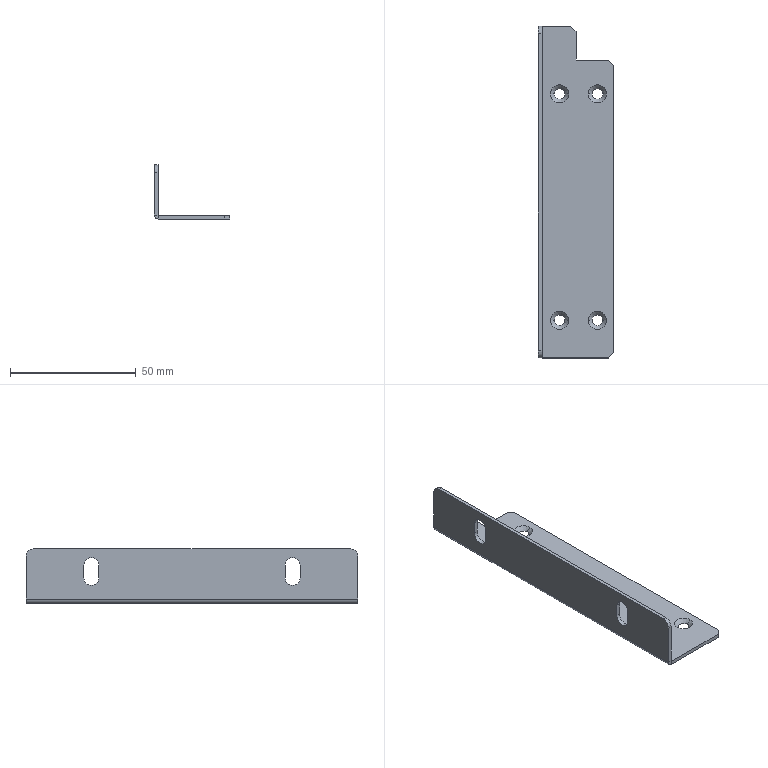Part | SolidWorks | features ICE 3, CornerTrim 2, Chamfer 1, EdgeFlange 1, FlatPattern 1, SMBaseFlange 1, SheetMetal 1 | 1 solid | 39 faces | box 30 x 132 x 21.5 mm | volume 9178 mm3 | plane 21 | cylinder 10 | cone 8 | commonest cylinder face diameters 6 x8 0.2 x1 3.2 x1
STEP:
#1=CARTESIAN_POINT('',(-8.6,39.,-1.5));
#2=VERTEX_POINT('',#1);
#3=CARTESIAN_POINT('',(-4.4,39.,-1.5));
#4=VERTEX_POINT('',#3);
#5=CARTESIAN_POINT('',(-6.5,39.,-1.5));
#6=DIRECTION('',(0.,0.,1.));
#7=DIRECTION('',(1.,0.,0.));
#8=AXIS2_PLACEMENT_3D('',#5,#6,#7);
#9=CIRCLE('',#8,2.1);
#10=EDGE_CURVE('',#2,#4,#9,.T.);
#11=ORIENTED_EDGE('',*,*,#10,.F.);
#12=CARTESIAN_POINT('',(-10.1,39.,0.));
#13=VERTEX_POINT('',#12);
#14=CARTESIAN_POINT('',(-8.6,39.,-1.5));
#15=DIRECTION('',(-0.7071,0.,0.7071));
#16=VECTOR('',#15,1000.);
#17=LINE('',#14,#16);
#18=EDGE_CURVE('',#2,#13,#17,.T.);
#19=ORIENTED_EDGE('',*,*,#18,.T.);
#20=CARTESIAN_POINT('',(-2.9,39.,0.));
#21=VERTEX_POINT('',#20);
#22=CARTESIAN_POINT('',(-6.5,39.,0.));
#23=DIRECTION('',(0.,0.,-1.));
#24=DIRECTION('',(1.,0.,0.));
#25=AXIS2_PLACEMENT_3D('',#22,#23,#24);
#26=CIRCLE('',#25,3.6);
#27=EDGE_CURVE('',#21,#13,#26,.T.);
#28=ORIENTED_EDGE('',*,*,#27,.F.);
#29=CARTESIAN_POINT('',(-4.4,39.,-1.5));
#30=DIRECTION('',(0.7071,0.,0.7071));
#31=VECTOR('',#30,1000.);
#32=LINE('',#29,#31);
#33=EDGE_CURVE('',#4,#21,#32,.T.);
#34=ORIENTED_EDGE('',*,*,#33,.F.);
#35=EDGE_LOOP('',(#11,#19,#28,#34));
#36=FACE_OUTER_BOUND('',#35,.T.);
#37=CARTESIAN_POINT('',(-6.5,39.,-1.5));
#38=DIRECTION('',(0.,0.,1.));
#39=DIRECTION('',(1.,0.,0.));
#40=AXIS2_PLACEMENT_3D('',#37,#38,#39);
#41=CONICAL_SURFACE('',#40,2.1,0.7854);
#42=ADVANCED_FACE('',(#36),#41,.F.);
#43=CARTESIAN_POINT('',(6.4,39.,-1.5));
#44=VERTEX_POINT('',#43);
#45=CARTESIAN_POINT('',(10.6,39.,-1.5));
#46=VERTEX_POINT('',#45);
#47=CARTESIAN_POINT('',(8.5,39.,-1.5));
#48=DIRECTION('',(0.,0.,1.));
#49=DIRECTION('',(1.,0.,0.));
#50=AXIS2_PLACEMENT_3D('',#47,#48,#49);
#51=CIRCLE('',#50,2.1);
#52=EDGE_CURVE('',#44,#46,#51,.T.);
#53=ORIENTED_EDGE('',*,*,#52,.F.);
#54=CARTESIAN_POINT('',(4.9,39.,0.));
#55=VERTEX_POINT('',#54);
#56=CARTESIAN_POINT('',(6.4,39.,-1.5));
#57=DIRECTION('',(-0.7071,0.,0.7071));
#58=VECTOR('',#57,1000.);
#59=LINE('',#56,#58);
#60=EDGE_CURVE('',#44,#55,#59,.T.);
#61=ORIENTED_EDGE('',*,*,#60,.T.);
#62=CARTESIAN_POINT('',(12.1,39.,0.));
#63=VERTEX_POINT('',#62);
#64=CARTESIAN_POINT('',(8.5,39.,0.));
#65=DIRECTION('',(0.,0.,-1.));
#66=DIRECTION('',(1.,0.,0.));
#67=AXIS2_PLACEMENT_3D('',#64,#65,#66);
#68=CIRCLE('',#67,3.6);
#69=EDGE_CURVE('',#63,#55,#68,.T.);
#70=ORIENTED_EDGE('',*,*,#69,.F.);
#71=CARTESIAN_POINT('',(10.6,39.,-1.5));
#72=DIRECTION('',(0.7071,0.,0.7071));
#73=VECTOR('',#72,1000.);
#74=LINE('',#71,#73);
#75=EDGE_CURVE('',#46,#63,#74,.T.);
#76=ORIENTED_EDGE('',*,*,#75,.F.);
#77=EDGE_LOOP('',(#53,#61,#70,#76));
#78=FACE_OUTER_BOUND('',#77,.T.);
#79=CARTESIAN_POINT('',(8.5,39.,-1.5));
#80=DIRECTION('',(0.,0.,1.));
#81=DIRECTION('',(1.,0.,0.));
#82=AXIS2_PLACEMENT_3D('',#79,#80,#81);
#83=CONICAL_SURFACE('',#82,2.1,0.7854);
#84=ADVANCED_FACE('',(#78),#83,.F.);
#85=CARTESIAN_POINT('',(6.4,-51.,-1.5));
#86=VERTEX_POINT('',#85);
#87=CARTESIAN_POINT('',(10.6,-51.,-1.5));
#88=VERTEX_POINT('',#87);
#89=CARTESIAN_POINT('',(8.5,-51.,-1.5));
#90=DIRECTION('',(0.,0.,1.));
#91=DIRECTION('',(1.,0.,0.));
#92=AXIS2_PLACEMENT_3D('',#89,#90,#91);
#93=CIRCLE('',#92,2.1);
#94=EDGE_CURVE('',#86,#88,#93,.T.);
#95=ORIENTED_EDGE('',*,*,#94,.F.);
#96=CARTESIAN_POINT('',(4.9,-51.,0.));
#97=VERTEX_POINT('',#96);
#98=CARTESIAN_POINT('',(6.4,-51.,-1.5));
#99=DIRECTION('',(-0.7071,0.,0.7071));
#100=VECTOR('',#99,1000.);
#101=LINE('',#98,#100);
#102=EDGE_CURVE('',#86,#97,#101,.T.);
#103=ORIENTED_EDGE('',*,*,#102,.T.);
#104=CARTESIAN_POINT('',(12.1,-51.,0.));
#105=VERTEX_POINT('',#104);
#106=CARTESIAN_POINT('',(8.5,-51.,0.));
#107=DIRECTION('',(0.,0.,-1.));
#108=DIRECTION('',(1.,0.,0.));
#109=AXIS2_PLACEMENT_3D('',#106,#107,#108);
#110=CIRCLE('',#109,3.6);
#111=EDGE_CURVE('',#105,#97,#110,.T.);
#112=ORIENTED_EDGE('',*,*,#111,.F.);
#113=CARTESIAN_POINT('',(10.6,-51.,-1.5));
#114=DIRECTION('',(0.7071,0.,0.7071));
#115=VECTOR('',#114,1000.);
#116=LINE('',#113,#115);
#117=EDGE_CURVE('',#88,#105,#116,.T.);
#118=ORIENTED_EDGE('',*,*,#117,.F.);
#119=EDGE_LOOP('',(#95,#103,#112,#118));
#120=FACE_OUTER_BOUND('',#119,.T.);
#121=CARTESIAN_POINT('',(8.5,-51.,-1.5));
#122=DIRECTION('',(0.,0.,1.));
#123=DIRECTION('',(1.,0.,0.));
#124=AXIS2_PLACEMENT_3D('',#121,#122,#123);
#125=CONICAL_SURFACE('',#124,2.1,0.7854);
#126=ADVANCED_FACE('',(#120),#125,.F.);
#127=CARTESIAN_POINT('',(-8.6,-51.,-1.5));
#128=VERTEX_POINT('',#127);
#129=CARTESIAN_POINT('',(-4.4,-51.,-1.5));
#130=VERTEX_POINT('',#129);
#131=CARTESIAN_POINT('',(-6.5,-51.,-1.5));
#132=DIRECTION('',(0.,0.,1.));
#133=DIRECTION('',(1.,0.,0.));
#134=AXIS2_PLACEMENT_3D('',#131,#132,#133);
#135=CIRCLE('',#134,2.1);
#136=EDGE_CURVE('',#128,#130,#135,.T.);
#137=ORIENTED_EDGE('',*,*,#136,.F.);
#138=CARTESIAN_POINT('',(-10.1,-51.,0.));
#139=VERTEX_POINT('',#138);
#140=CARTESIAN_POINT('',(-8.6,-51.,-1.5));
#141=DIRECTION('',(-0.7071,0.,0.7071));
#142=VECTOR('',#141,1000.);
#143=LINE('',#140,#142);
#144=EDGE_CURVE('',#128,#139,#143,.T.);
#145=ORIENTED_EDGE('',*,*,#144,.T.);
#146=CARTESIAN_POINT('',(-2.9,-51.,0.));
#147=VERTEX_POINT('',#146);
#148=CARTESIAN_POINT('',(-6.5,-51.,0.));
#149=DIRECTION('',(0.,0.,-1.));
#150=DIRECTION('',(1.,0.,0.));
#151=AXIS2_PLACEMENT_3D('',#148,#149,#150);
#152=CIRCLE('',#151,3.6);
#153=EDGE_CURVE('',#147,#139,#152,.T.);
#154=ORIENTED_EDGE('',*,*,#153,.F.);
#155=CARTESIAN_POINT('',(-4.4,-51.,-1.5));
#156=DIRECTION('',(0.7071,0.,0.7071));
#157=VECTOR('',#156,1000.);
#158=LINE('',#155,#157);
#159=EDGE_CURVE('',#130,#147,#158,.T.);
#160=ORIENTED_EDGE('',*,*,#159,.F.);
#161=EDGE_LOOP('',(#137,#145,#154,#160));
#162=FACE_OUTER_BOUND('',#161,.T.);
#163=CARTESIAN_POINT('',(-6.5,-51.,-1.5));
#164=DIRECTION('',(0.,0.,1.));
#165=DIRECTION('',(1.,0.,0.));
#166=AXIS2_PLACEMENT_3D('',#163,#164,#165);
#167=CONICAL_SURFACE('',#166,2.1,0.7854);
#168=ADVANCED_FACE('',(#162),#167,.F.);
#169=CARTESIAN_POINT('',(-13.5,43.,13.5));
#170=VERTEX_POINT('',#169);
#171=CARTESIAN_POINT('',(-13.5,40.,16.5));
#172=VERTEX_POINT('',#171);
#173=CARTESIAN_POINT('',(-13.5,40.,13.5));
#174=DIRECTION('',(1.,0.,0.));
#175=DIRECTION('',(0.,0.,-1.));
#176=AXIS2_PLACEMENT_3D('',#173,#174,#175);
#177=CIRCLE('',#176,3.);
#178=EDGE_CURVE('',#170,#172,#177,.T.);
#179=ORIENTED_EDGE('',*,*,#178,.T.);
#180=CARTESIAN_POINT('',(-15.,40.,16.5));
#181=VERTEX_POINT('',#180);
#182=CARTESIAN_POINT('',(-5.,40.,16.5));
#183=DIRECTION('',(-1.,0.,0.));
#184=VECTOR('',#183,1000.);
#185=LINE('',#182,#184);
#186=EDGE_CURVE('',#172,#181,#185,.T.);
#187=ORIENTED_EDGE('',*,*,#186,.T.);
#188=CARTESIAN_POINT('',(-15.,43.,13.5));
#189=VERTEX_POINT('',#188);
#190=CARTESIAN_POINT('',(-15.,40.,13.5));
#191=DIRECTION('',(-1.,0.,0.));
#192=DIRECTION('',(0.,0.,1.));
#193=AXIS2_PLACEMENT_3D('',#190,#191,#192);
#194=CIRCLE('',#193,3.);
#195=EDGE_CURVE('',#181,#189,#194,.T.);
#196=ORIENTED_EDGE('',*,*,#195,.T.);
#197=CARTESIAN_POINT('',(-5.,43.,13.5));
#198=DIRECTION('',(-1.,0.,0.));
#199=VECTOR('',#198,1000.);
#200=LINE('',#197,#199);
#201=EDGE_CURVE('',#170,#189,#200,.T.);
#202=ORIENTED_EDGE('',*,*,#201,.F.);
#203=EDGE_LOOP('',(#179,#187,#196,#202));
#204=FACE_OUTER_BOUND('',#203,.T.);
#205=CARTESIAN_POINT('',(-5.,40.,13.5));
#206=DIRECTION('',(-1.,0.,0.));
#207=DIRECTION('',(0.,0.,1.));
#208=AXIS2_PLACEMENT_3D('',#205,#206,#207);
#209=CYLINDRICAL_SURFACE('',#208,3.);
#210=ADVANCED_FACE('',(#204),#209,.F.);
#211=CARTESIAN_POINT('',(-13.5,-37.,13.5));
#212=VERTEX_POINT('',#211);
#213=CARTESIAN_POINT('',(-13.5,-40.,16.5));
#214=VERTEX_POINT('',#213);
#215=CARTESIAN_POINT('',(-13.5,-40.,13.5));
#216=DIRECTION('',(1.,0.,0.));
#217=DIRECTION('',(0.,0.,-1.));
#218=AXIS2_PLACEMENT_3D('',#215,#216,#217);
#219=CIRCLE('',#218,3.);
#220=EDGE_CURVE('',#212,#214,#219,.T.);
#221=ORIENTED_EDGE('',*,*,#220,.T.);
#222=CARTESIAN_POINT('',(-15.,-40.,16.5));
#223=VERTEX_POINT('',#222);
#224=CARTESIAN_POINT('',(-5.,-40.,16.5));
#225=DIRECTION('',(-1.,0.,0.));
#226=VECTOR('',#225,1000.);
#227=LINE('',#224,#226);
#228=EDGE_CURVE('',#214,#223,#227,.T.);
#229=ORIENTED_EDGE('',*,*,#228,.T.);
#230=CARTESIAN_POINT('',(-15.,-37.,13.5));
#231=VERTEX_POINT('',#230);
#232=CARTESIAN_POINT('',(-15.,-40.,13.5));
#233=DIRECTION('',(-1.,0.,0.));
#234=DIRECTION('',(0.,0.,1.));
#235=AXIS2_PLACEMENT_3D('',#232,#233,#234);
#236=CIRCLE('',#235,3.);
#237=EDGE_CURVE('',#223,#231,#236,.T.);
#238=ORIENTED_EDGE('',*,*,#237,.T.);
#239=CARTESIAN_POINT('',(-5.,-37.,13.5));
#240=DIRECTION('',(-1.,0.,0.));
#241=VECTOR('',#240,1000.);
#242=LINE('',#239,#241);
#243=EDGE_CURVE('',#212,#231,#242,.T.);
#244=ORIENTED_EDGE('',*,*,#243,.F.);
#245=EDGE_LOOP('',(#221,#229,#238,#244));
#246=FACE_OUTER_BOUND('',#245,.T.);
#247=CARTESIAN_POINT('',(-5.,-40.,13.5));
#248=DIRECTION('',(-1.,0.,0.));
#249=DIRECTION('',(0.,0.,1.));
#250=AXIS2_PLACEMENT_3D('',#247,#248,#249);
#251=CYLINDRICAL_SURFACE('',#250,3.);
#252=ADVANCED_FACE('',(#246),#251,.F.);
#253=CARTESIAN_POINT('',(-13.4,-66.,-1.5));
#254=VERTEX_POINT('',#253);
#255=CARTESIAN_POINT('',(13.,-66.,-1.5));
#256=VERTEX_POINT('',#255);
#257=CARTESIAN_POINT('',(-15.,-66.,-1.5));
#258=DIRECTION('',(1.,0.,0.));
#259=VECTOR('',#258,1000.);
#260=LINE('',#257,#259);
#261=EDGE_CURVE('',#254,#256,#260,.T.);
#262=ORIENTED_EDGE('',*,*,#261,.T.);
#263=CARTESIAN_POINT('',(13.,-66.,0.));
#264=VERTEX_POINT('',#263);
#265=CARTESIAN_POINT('',(13.,-66.,-1.5));
#266=DIRECTION('',(0.,0.,1.));
#267=VECTOR('',#266,1000.);
#268=LINE('',#265,#267);
#269=EDGE_CURVE('',#256,#264,#268,.T.);
#270=ORIENTED_EDGE('',*,*,#269,.T.);
#271=CARTESIAN_POINT('',(-13.4,-66.,0.));
#272=VERTEX_POINT('',#271);
#273=CARTESIAN_POINT('',(-15.,-66.,0.));
#274=DIRECTION('',(1.,0.,0.));
#275=VECTOR('',#274,1000.);
#276=LINE('',#273,#275);
#277=EDGE_CURVE('',#272,#264,#276,.T.);
#278=ORIENTED_EDGE('',*,*,#277,.F.);
#279=CARTESIAN_POINT('',(-13.4,-66.,0.));
#280=DIRECTION('',(0.,0.,-1.));
#281=VECTOR('',#280,1000.);
#282=LINE('',#279,#281);
#283=EDGE_CURVE('',#272,#254,#282,.T.);
#284=ORIENTED_EDGE('',*,*,#283,.T.);
#285=EDGE_LOOP('',(#262,#270,#278,#284));
#286=FACE_OUTER_BOUND('',#285,.T.);
#287=CARTESIAN_POINT('',(-15.,-66.,-1.5));
#288=DIRECTION('',(0.,-1.,0.));
#289=DIRECTION('',(0.,0.,-1.));
#290=AXIS2_PLACEMENT_3D('',#287,#288,#289);
#291=PLANE('',#290);
#292=ADVANCED_FACE('',(#286),#291,.T.);
#293=CARTESIAN_POINT('',(-6.5,-51.,-1.5));
#294=DIRECTION('',(0.,0.,1.));
#295=DIRECTION('',(1.,0.,0.));
#296=AXIS2_PLACEMENT_3D('',#293,#294,#295);
#297=CIRCLE('',#296,2.1);
#298=EDGE_CURVE('',#130,#128,#297,.T.);
#299=ORIENTED_EDGE('',*,*,#298,.T.);
#300=ORIENTED_EDGE('',*,*,#136,.T.);
#301=EDGE_LOOP('',(#299,#300));
#302=FACE_BOUND('',#301,.T.);
#303=CARTESIAN_POINT('',(8.5,-51.,-1.5));
#304=DIRECTION('',(0.,0.,1.));
#305=DIRECTION('',(1.,0.,0.));
#306=AXIS2_PLACEMENT_3D('',#303,#304,#305);
#307=CIRCLE('',#306,2.1);
#308=EDGE_CURVE('',#88,#86,#307,.T.);
#309=ORIENTED_EDGE('',*,*,#308,.T.);
#310=ORIENTED_EDGE('',*,*,#94,.T.);
#311=EDGE_LOOP('',(#309,#310));
#312=FACE_BOUND('',#311,.T.);
#313=CARTESIAN_POINT('',(8.5,39.,-1.5));
#314=DIRECTION('',(0.,0.,1.));
#315=DIRECTION('',(1.,0.,0.));
#316=AXIS2_PLACEMENT_3D('',#313,#314,#315);
#317=CIRCLE('',#316,2.1);
#318=EDGE_CURVE('',#46,#44,#317,.T.);
#319=ORIENTED_EDGE('',*,*,#318,.T.);
#320=ORIENTED_EDGE('',*,*,#52,.T.);
#321=EDGE_LOOP('',(#319,#320));
#322=FACE_BOUND('',#321,.T.);
#323=CARTESIAN_POINT('',(-6.5,39.,-1.5));
#324=DIRECTION('',(0.,0.,1.));
#325=DIRECTION('',(1.,0.,0.));
#326=AXIS2_PLACEMENT_3D('',#323,#324,#325);
#327=CIRCLE('',#326,2.1);
#328=EDGE_CURVE('',#4,#2,#327,.T.);
#329=ORIENTED_EDGE('',*,*,#328,.T.);
#330=ORIENTED_EDGE('',*,*,#10,.T.);
#331=EDGE_LOOP('',(#329,#330));
#332=FACE_BOUND('',#331,.T.);
#333=CARTESIAN_POINT('',(0.,52.5,-1.5));
#334=VERTEX_POINT('',#333);
#335=CARTESIAN_POINT('',(13.,52.5,-1.5));
#336=VERTEX_POINT('',#335);
#337=CARTESIAN_POINT('',(0.,52.5,-1.5));
#338=DIRECTION('',(1.,0.,0.));
#339=VECTOR('',#338,1000.);
#340=LINE('',#337,#339);
#341=EDGE_CURVE('',#334,#336,#340,.T.);
#342=ORIENTED_EDGE('',*,*,#341,.T.);
#343=CARTESIAN_POINT('',(15.,50.5,-1.5));
#344=VERTEX_POINT('',#343);
#345=CARTESIAN_POINT('',(15.,50.5,-1.5));
#346=DIRECTION('',(0.7071,-0.7071,0.));
#347=VECTOR('',#346,1000.);
#348=LINE('',#345,#347);
#349=EDGE_CURVE('',#336,#344,#348,.T.);
#350=ORIENTED_EDGE('',*,*,#349,.T.);
#351=CARTESIAN_POINT('',(15.,-64.,-1.5));
#352=VERTEX_POINT('',#351);
#353=CARTESIAN_POINT('',(15.,66.,-1.5));
#354=DIRECTION('',(0.,1.,0.));
#355=VECTOR('',#354,1000.);
#356=LINE('',#353,#355);
#357=EDGE_CURVE('',#352,#344,#356,.T.);
#358=ORIENTED_EDGE('',*,*,#357,.F.);
#359=CARTESIAN_POINT('',(13.,-66.,-1.5));
#360=DIRECTION('',(-0.7071,-0.7071,0.));
#361=VECTOR('',#360,1000.);
#362=LINE('',#359,#361);
#363=EDGE_CURVE('',#352,#256,#362,.T.);
#364=ORIENTED_EDGE('',*,*,#363,.T.);
#365=ORIENTED_EDGE('',*,*,#261,.F.);
#366=CARTESIAN_POINT('',(-13.4,66.,-1.5));
#367=VERTEX_POINT('',#366);
#368=CARTESIAN_POINT('',(-13.4,-66.,-1.5));
#369=DIRECTION('',(0.,1.,0.));
#370=VECTOR('',#369,1000.);
#371=LINE('',#368,#370);
#372=EDGE_CURVE('',#254,#367,#371,.T.);
#373=ORIENTED_EDGE('',*,*,#372,.T.);
#374=CARTESIAN_POINT('',(-2.,66.,-1.5));
#375=VERTEX_POINT('',#374);
#376=CARTESIAN_POINT('',(-15.,66.,-1.5));
#377=DIRECTION('',(-1.,0.,0.));
#378=VECTOR('',#377,1000.);
#379=LINE('',#376,#378);
#380=EDGE_CURVE('',#375,#367,#379,.T.);
#381=ORIENTED_EDGE('',*,*,#380,.F.);
#382=CARTESIAN_POINT('',(0.,64.,-1.5));
#383=VERTEX_POINT('',#382);
#384=CARTESIAN_POINT('',(0.,64.,-1.5));
#385=DIRECTION('',(0.7071,-0.7071,0.));
#386=VECTOR('',#385,1000.);
#387=LINE('',#384,#386);
#388=EDGE_CURVE('',#375,#383,#387,.T.);
#389=ORIENTED_EDGE('',*,*,#388,.T.);
#390=CARTESIAN_POINT('',(0.,0.,-1.5));
#391=DIRECTION('',(0.,-1.,0.));
#392=VECTOR('',#391,1000.);
#393=LINE('',#390,#392);
#394=EDGE_CURVE('',#383,#334,#393,.T.);
#395=ORIENTED_EDGE('',*,*,#394,.T.);
#396=EDGE_LOOP('',(#342,#350,#358,#364,#365,#373,#381,#389,#395));
#397=FACE_OUTER_BOUND('',#396,.T.);
#398=CARTESIAN_POINT('',(0.,0.,-1.5));
#399=DIRECTION('',(0.,0.,1.));
#400=DIRECTION('',(1.,0.,0.));
#401=AXIS2_PLACEMENT_3D('',#398,#399,#400);
#402=PLANE('',#401);
#403=ADVANCED_FACE('',(#302,#312,#322,#332,#397),#402,.F.);
#404=ORIENTED_EDGE('',*,*,#153,.T.);
#405=CARTESIAN_POINT('',(-6.5,-51.,0.));
#406=DIRECTION('',(0.,0.,-1.));
#407=DIRECTION('',(1.,0.,0.));
#408=AXIS2_PLACEMENT_3D('',#405,#406,#407);
#409=CIRCLE('',#408,3.6);
#410=EDGE_CURVE('',#139,#147,#409,.T.);
#411=ORIENTED_EDGE('',*,*,#410,.T.);
#412=EDGE_LOOP('',(#404,#411));
#413=FACE_BOUND('',#412,.T.);
#414=ORIENTED_EDGE('',*,*,#111,.T.);
#415=CARTESIAN_POINT('',(8.5,-51.,0.));
#416=DIRECTION('',(0.,0.,-1.));
#417=DIRECTION('',(1.,0.,0.));
#418=AXIS2_PLACEMENT_3D('',#415,#416,#417);
#419=CIRCLE('',#418,3.6);
#420=EDGE_CURVE('',#97,#105,#419,.T.);
#421=ORIENTED_EDGE('',*,*,#420,.T.);
#422=EDGE_LOOP('',(#414,#421));
#423=FACE_BOUND('',#422,.T.);
#424=ORIENTED_EDGE('',*,*,#69,.T.);
#425=CARTESIAN_POINT('',(8.5,39.,0.));
#426=DIRECTION('',(0.,0.,-1.));
#427=DIRECTION('',(1.,0.,0.));
#428=AXIS2_PLACEMENT_3D('',#425,#426,#427);
#429=CIRCLE('',#428,3.6);
#430=EDGE_CURVE('',#55,#63,#429,.T.);
#431=ORIENTED_EDGE('',*,*,#430,.T.);
#432=EDGE_LOOP('',(#424,#431));
#433=FACE_BOUND('',#432,.T.);
#434=ORIENTED_EDGE('',*,*,#27,.T.);
#435=CARTESIAN_POINT('',(-6.5,39.,0.));
#436=DIRECTION('',(0.,0.,-1.));
#437=DIRECTION('',(1.,0.,0.));
#438=AXIS2_PLACEMENT_3D('',#435,#436,#437);
#439=CIRCLE('',#438,3.6);
#440=EDGE_CURVE('',#13,#21,#439,.T.);
#441=ORIENTED_EDGE('',*,*,#440,.T.);
#442=EDGE_LOOP('',(#434,#441));
#443=FACE_BOUND('',#442,.T.);
#444=CARTESIAN_POINT('',(15.,-64.,0.));
#445=VERTEX_POINT('',#444);
#446=CARTESIAN_POINT('',(15.,50.5,0.));
#447=VERTEX_POINT('',#446);
#448=CARTESIAN_POINT('',(15.,66.,0.));
#449=DIRECTION('',(0.,1.,0.));
#450=VECTOR('',#449,1000.);
#451=LINE('',#448,#450);
#452=EDGE_CURVE('',#445,#447,#451,.T.);
#453=ORIENTED_EDGE('',*,*,#452,.T.);
#454=CARTESIAN_POINT('',(13.,52.5,0.));
#455=VERTEX_POINT('',#454);
#456=CARTESIAN_POINT('',(32.75,32.75,0.));
#457=DIRECTION('',(-0.7071,0.7071,0.));
#458=VECTOR('',#457,1000.);
#459=LINE('',#456,#458);
#460=EDGE_CURVE('',#447,#455,#459,.T.);
#461=ORIENTED_EDGE('',*,*,#460,.T.);
#462=CARTESIAN_POINT('',(0.,52.5,0.));
#463=VERTEX_POINT('',#462);
#464=CARTESIAN_POINT('',(15.,52.5,0.));
#465=DIRECTION('',(1.,0.,0.));
#466=VECTOR('',#465,1000.);
#467=LINE('',#464,#466);
#468=EDGE_CURVE('',#463,#455,#467,.T.);
#469=ORIENTED_EDGE('',*,*,#468,.F.);
#470=CARTESIAN_POINT('',(0.,64.,0.));
#471=VERTEX_POINT('',#470);
#472=CARTESIAN_POINT('',(0.,66.,0.));
#473=DIRECTION('',(0.,-1.,0.));
#474=VECTOR('',#473,1000.);
#475=LINE('',#472,#474);
#476=EDGE_CURVE('',#471,#463,#475,.T.);
#477=ORIENTED_EDGE('',*,*,#476,.F.);
#478=CARTESIAN_POINT('',(-2.,66.,0.));
#479=VERTEX_POINT('',#478);
#480=CARTESIAN_POINT('',(32.,32.,0.));
#481=DIRECTION('',(-0.7071,0.7071,0.));
#482=VECTOR('',#481,1000.);
#483=LINE('',#480,#482);
#484=EDGE_CURVE('',#471,#479,#483,.T.);
#485=ORIENTED_EDGE('',*,*,#484,.T.);
#486=CARTESIAN_POINT('',(-13.4,66.,0.));
#487=VERTEX_POINT('',#486);
#488=CARTESIAN_POINT('',(-15.,66.,0.));
#489=DIRECTION('',(-1.,0.,0.));
#490=VECTOR('',#489,1000.);
#491=LINE('',#488,#490);
#492=EDGE_CURVE('',#479,#487,#491,.T.);
#493=ORIENTED_EDGE('',*,*,#492,.T.);
#494=CARTESIAN_POINT('',(-13.4,-66.,0.));
#495=DIRECTION('',(0.,1.,0.));
#496=VECTOR('',#495,1000.);
#497=LINE('',#494,#496);
#498=EDGE_CURVE('',#272,#487,#497,.T.);
#499=ORIENTED_EDGE('',*,*,#498,.F.);
#500=ORIENTED_EDGE('',*,*,#277,.T.);
#501=CARTESIAN_POINT('',(39.5,-39.5,0.));
#502=DIRECTION('',(0.7071,0.7071,0.));
#503=VECTOR('',#502,1000.);
#504=LINE('',#501,#503);
#505=EDGE_CURVE('',#264,#445,#504,.T.);
#506=ORIENTED_EDGE('',*,*,#505,.T.);
#507=EDGE_LOOP('',(#453,#461,#469,#477,#485,#493,#499,#500,#506));
#508=FACE_OUTER_BOUND('',#507,.T.);
#509=CARTESIAN_POINT('',(0.,0.,0.));
#510=DIRECTION('',(0.,0.,1.));
#511=DIRECTION('',(1.,0.,0.));
#512=AXIS2_PLACEMENT_3D('',#509,#510,#511);
#513=PLANE('',#512);
#514=ADVANCED_FACE('',(#413,#423,#433,#443,#508),#513,.T.);
#515=ORIENTED_EDGE('',*,*,#357,.T.);
#516=CARTESIAN_POINT('',(15.,50.5,0.));
#517=DIRECTION('',(0.,0.,1.));
#518=VECTOR('',#517,1000.);
#519=LINE('',#516,#518);
#520=EDGE_CURVE('',#344,#447,#519,.T.);
#521=ORIENTED_EDGE('',*,*,#520,.T.);
#522=ORIENTED_EDGE('',*,*,#452,.F.);
#523=CARTESIAN_POINT('',(15.,-64.,-1.5));
#524=DIRECTION('',(0.,0.,-1.));
#525=VECTOR('',#524,1000.);
#526=LINE('',#523,#525);
#527=EDGE_CURVE('',#445,#352,#526,.T.);
#528=ORIENTED_EDGE('',*,*,#527,.T.);
#529=EDGE_LOOP('',(#515,#521,#522,#528));
#530=FACE_OUTER_BOUND('',#529,.T.);
#531=CARTESIAN_POINT('',(15.,66.,-1.5));
#532=DIRECTION('',(1.,0.,0.));
#533=DIRECTION('',(0.,1.,0.));
#534=AXIS2_PLACEMENT_3D('',#531,#532,#533);
#535=PLANE('',#534);
#536=ADVANCED_FACE('',(#530),#535,.T.);
#537=ORIENTED_EDGE('',*,*,#492,.F.);
#538=CARTESIAN_POINT('',(-2.,66.,-1.5));
#539=DIRECTION('',(0.,0.,-1.));
#540=VECTOR('',#539,1000.);
#541=LINE('',#538,#540);
#542=EDGE_CURVE('',#479,#375,#541,.T.);
#543=ORIENTED_EDGE('',*,*,#542,.T.);
#544=ORIENTED_EDGE('',*,*,#380,.T.);
#545=CARTESIAN_POINT('',(-13.4,66.,0.));
#546=DIRECTION('',(0.,0.,-1.));
#547=VECTOR('',#546,1000.);
#548=LINE('',#545,#547);
#549=EDGE_CURVE('',#487,#367,#548,.T.);
#550=ORIENTED_EDGE('',*,*,#549,.F.);
#551=EDGE_LOOP('',(#537,#543,#544,#550));
#552=FACE_OUTER_BOUND('',#551,.T.);
#553=CARTESIAN_POINT('',(-15.,66.,-1.5));
#554=DIRECTION('',(0.,1.,0.));
#555=DIRECTION('',(0.,0.,1.));
#556=AXIS2_PLACEMENT_3D('',#553,#554,#555);
#557=PLANE('',#556);
#558=ADVANCED_FACE('',(#552),#557,.T.);
#559=CARTESIAN_POINT('',(-13.5,66.,0.1));
#560=VERTEX_POINT('',#559);
#561=CARTESIAN_POINT('',(-15.,66.,0.1));
#562=VERTEX_POINT('',#561);
#563=CARTESIAN_POINT('',(-15.,66.,0.1));
#564=DIRECTION('',(-1.,0.,0.));
#565=VECTOR('',#564,1000.);
#566=LINE('',#563,#565);
#567=EDGE_CURVE('',#560,#562,#566,.T.);
#568=ORIENTED_EDGE('',*,*,#567,.F.);
#569=CARTESIAN_POINT('',(-13.4,66.,0.1));
#570=DIRECTION('',(0.,1.,0.));
#571=DIRECTION('',(0.,0.,-1.));
#572=AXIS2_PLACEMENT_3D('',#569,#570,#571);
#573=CIRCLE('',#572,0.1);
#574=EDGE_CURVE('',#487,#560,#573,.T.);
#575=ORIENTED_EDGE('',*,*,#574,.F.);
#576=ORIENTED_EDGE('',*,*,#549,.T.);
#577=CARTESIAN_POINT('',(-13.4,66.,0.1));
#578=DIRECTION('',(0.,1.,0.));
#579=DIRECTION('',(0.,0.,-1.));
#580=AXIS2_PLACEMENT_3D('',#577,#578,#579);
#581=CIRCLE('',#580,1.6);
#582=EDGE_CURVE('',#367,#562,#581,.T.);
#583=ORIENTED_EDGE('',*,*,#582,.T.);
#584=EDGE_LOOP('',(#568,#575,#576,#583));
#585=FACE_OUTER_BOUND('',#584,.T.);
#586=CARTESIAN_POINT('',(-13.4,66.,0.1));
#587=DIRECTION('',(0.,1.,0.));
#588=DIRECTION('',(0.,0.,1.));
#589=AXIS2_PLACEMENT_3D('',#586,#587,#588);
#590=PLANE('',#589);
#591=ADVANCED_FACE('',(#585),#590,.T.);
#592=CARTESIAN_POINT('',(-13.5,-66.,0.1));
#593=VERTEX_POINT('',#592);
#594=CARTESIAN_POINT('',(-13.4,-66.,0.1));
#595=DIRECTION('',(0.,-1.,0.));
#596=DIRECTION('',(0.,0.,-1.));
#597=AXIS2_PLACEMENT_3D('',#594,#595,#596);
#598=CIRCLE('',#597,0.1);
#599=EDGE_CURVE('',#593,#272,#598,.T.);
#600=ORIENTED_EDGE('',*,*,#599,.F.);
#601=CARTESIAN_POINT('',(-15.,-66.,0.1));
#602=VERTEX_POINT('',#601);
#603=CARTESIAN_POINT('',(-13.5,-66.,0.1));
#604=DIRECTION('',(-1.,0.,0.));
#605=VECTOR('',#604,1000.);
#606=LINE('',#603,#605);
#607=EDGE_CURVE('',#593,#602,#606,.T.);
#608=ORIENTED_EDGE('',*,*,#607,.T.);
#609=CARTESIAN_POINT('',(-13.4,-66.,0.1));
#610=DIRECTION('',(0.,-1.,0.));
#611=DIRECTION('',(0.,0.,-1.));
#612=AXIS2_PLACEMENT_3D('',#609,#610,#611);
#613=CIRCLE('',#612,1.6);
#614=EDGE_CURVE('',#602,#254,#613,.T.);
#615=ORIENTED_EDGE('',*,*,#614,.T.);
#616=ORIENTED_EDGE('',*,*,#283,.F.);
#617=EDGE_LOOP('',(#600,#608,#615,#616));
#618=FACE_OUTER_BOUND('',#617,.T.);
#619=CARTESIAN_POINT('',(-13.4,-66.,0.1));
#620=DIRECTION('',(0.,1.,0.));
#621=DIRECTION('',(0.,0.,1.));
#622=AXIS2_PLACEMENT_3D('',#619,#620,#621);
#623=PLANE('',#622);
#624=ADVANCED_FACE('',(#618),#623,.F.);
#625=ORIENTED_EDGE('',*,*,#372,.F.);
#626=ORIENTED_EDGE('',*,*,#614,.F.);
#627=CARTESIAN_POINT('',(-15.,66.,0.1));
#628=DIRECTION('',(0.,1.,0.));
#629=VECTOR('',#628,1000.);
#630=LINE('',#627,#629);
#631=EDGE_CURVE('',#602,#562,#630,.T.);
#632=ORIENTED_EDGE('',*,*,#631,.T.);
#633=ORIENTED_EDGE('',*,*,#582,.F.);
#634=EDGE_LOOP('',(#625,#626,#632,#633));
#635=FACE_OUTER_BOUND('',#634,.T.);
#636=CARTESIAN_POINT('',(-13.4,-66.,0.1));
#637=DIRECTION('',(0.,-1.,0.));
#638=DIRECTION('',(-1.,0.,0.));
#639=AXIS2_PLACEMENT_3D('',#636,#637,#638);
#640=CYLINDRICAL_SURFACE('',#639,1.6);
#641=ADVANCED_FACE('',(#635),#640,.T.);
#642=ORIENTED_EDGE('',*,*,#498,.T.);
#643=ORIENTED_EDGE('',*,*,#574,.T.);
#644=CARTESIAN_POINT('',(-13.5,66.,0.1));
#645=DIRECTION('',(0.,-1.,0.));
#646=VECTOR('',#645,1000.);
#647=LINE('',#644,#646);
#648=EDGE_CURVE('',#560,#593,#647,.T.);
#649=ORIENTED_EDGE('',*,*,#648,.T.);
#650=ORIENTED_EDGE('',*,*,#599,.T.);
#651=EDGE_LOOP('',(#642,#643,#649,#650));
#652=FACE_OUTER_BOUND('',#651,.T.);
#653=CARTESIAN_POINT('',(-13.4,-66.,0.1));
#654=DIRECTION('',(0.,-1.,0.));
#655=DIRECTION('',(-1.,0.,0.));
#656=AXIS2_PLACEMENT_3D('',#653,#654,#655);
#657=CYLINDRICAL_SURFACE('',#656,0.1);
#658=ADVANCED_FACE('',(#652),#657,.F.);
#659=CARTESIAN_POINT('',(-15.,66.,17.));
#660=VERTEX_POINT('',#659);
#661=CARTESIAN_POINT('',(-15.,66.,0.));
#662=DIRECTION('',(0.,0.,-1.));
#663=VECTOR('',#662,1000.);
#664=LINE('',#661,#663);
#665=EDGE_CURVE('',#660,#562,#664,.T.);
#666=ORIENTED_EDGE('',*,*,#665,.F.);
#667=CARTESIAN_POINT('',(-13.5,66.,17.));
#668=VERTEX_POINT('',#667);
#669=CARTESIAN_POINT('',(-15.,66.,17.));
#670=DIRECTION('',(1.,0.,0.));
#671=VECTOR('',#670,1000.);
#672=LINE('',#669,#671);
#673=EDGE_CURVE('',#660,#668,#672,.T.);
#674=ORIENTED_EDGE('',*,*,#673,.T.);
#675=CARTESIAN_POINT('',(-13.5,66.,0.));
#676=DIRECTION('',(0.,0.,-1.));
#677=VECTOR('',#676,1000.);
#678=LINE('',#675,#677);
#679=EDGE_CURVE('',#668,#560,#678,.T.);
#680=ORIENTED_EDGE('',*,*,#679,.T.);
#681=ORIENTED_EDGE('',*,*,#567,.T.);
#682=EDGE_LOOP('',(#666,#674,#680,#681));
#683=FACE_OUTER_BOUND('',#682,.T.);
#684=CARTESIAN_POINT('',(-15.,66.,0.));
#685=DIRECTION('',(0.,-1.,0.));
#686=DIRECTION('',(1.,0.,0.));
#687=AXIS2_PLACEMENT_3D('',#684,#685,#686);
#688=PLANE('',#687);
#689=ADVANCED_FACE('',(#683),#688,.F.);
#690=CARTESIAN_POINT('',(-13.5,-66.,17.));
#691=VERTEX_POINT('',#690);
#692=CARTESIAN_POINT('',(-13.5,-66.,20.));
#693=DIRECTION('',(0.,0.,1.));
#694=VECTOR('',#693,1000.);
#695=LINE('',#692,#694);
#696=EDGE_CURVE('',#593,#691,#695,.T.);
#697=ORIENTED_EDGE('',*,*,#696,.T.);
#698=CARTESIAN_POINT('',(-15.,-66.,17.));
#699=VERTEX_POINT('',#698);
#700=CARTESIAN_POINT('',(-15.,-66.,17.));
#701=DIRECTION('',(-1.,0.,0.));
#702=VECTOR('',#701,1000.);
#703=LINE('',#700,#702);
#704=EDGE_CURVE('',#691,#699,#703,.T.);
#705=ORIENTED_EDGE('',*,*,#704,.T.);
#706=CARTESIAN_POINT('',(-15.,-66.,0.));
#707=DIRECTION('',(0.,0.,1.));
#708=VECTOR('',#707,1000.);
#709=LINE('',#706,#708);
#710=EDGE_CURVE('',#602,#699,#709,.T.);
#711=ORIENTED_EDGE('',*,*,#710,.F.);
#712=ORIENTED_EDGE('',*,*,#607,.F.);
#713=EDGE_LOOP('',(#697,#705,#711,#712));
#714=FACE_OUTER_BOUND('',#713,.T.);
#715=CARTESIAN_POINT('',(-15.,-66.,20.));
#716=DIRECTION('',(0.,1.,0.));
#717=DIRECTION('',(-1.,0.,0.));
#718=AXIS2_PLACEMENT_3D('',#715,#716,#717);
#719=PLANE('',#718);
#720=ADVANCED_FACE('',(#714),#719,.F.);
#721=CARTESIAN_POINT('',(-15.,37.,8.5));
#722=VERTEX_POINT('',#721);
#723=CARTESIAN_POINT('',(-15.,37.,13.5));
#724=VERTEX_POINT('',#723);
#725=CARTESIAN_POINT('',(-15.,37.,8.5));
#726=DIRECTION('',(0.,0.,1.));
#727=VECTOR('',#726,1000.);
#728=LINE('',#725,#727);
#729=EDGE_CURVE('',#722,#724,#728,.T.);
#730=ORIENTED_EDGE('',*,*,#729,.F.);
#731=CARTESIAN_POINT('',(-15.,43.,8.5));
#732=VERTEX_POINT('',#731);
#733=CARTESIAN_POINT('',(-15.,40.,8.5));
#734=DIRECTION('',(-1.,0.,0.));
#735=DIRECTION('',(0.,0.,1.));
#736=AXIS2_PLACEMENT_3D('',#733,#734,#735);
#737=CIRCLE('',#736,3.);
#738=EDGE_CURVE('',#732,#722,#737,.T.);
#739=ORIENTED_EDGE('',*,*,#738,.F.);
#740=CARTESIAN_POINT('',(-15.,43.,8.5));
#741=DIRECTION('',(0.,0.,-1.));
#742=VECTOR('',#741,1000.);
#743=LINE('',#740,#742);
#744=EDGE_CURVE('',#189,#732,#743,.T.);
#745=ORIENTED_EDGE('',*,*,#744,.F.);
#746=ORIENTED_EDGE('',*,*,#195,.F.);
#747=CARTESIAN_POINT('',(-15.,40.,13.5));
#748=DIRECTION('',(-1.,0.,0.));
#749=DIRECTION('',(0.,0.,1.));
#750=AXIS2_PLACEMENT_3D('',#747,#748,#749);
#751=CIRCLE('',#750,3.);
#752=EDGE_CURVE('',#724,#181,#751,.T.);
#753=ORIENTED_EDGE('',*,*,#752,.F.);
#754=EDGE_LOOP('',(#730,#739,#745,#746,#753));
#755=FACE_BOUND('',#754,.T.);
#756=CARTESIAN_POINT('',(-15.,-43.,8.5));
#757=VERTEX_POINT('',#756);
#758=CARTESIAN_POINT('',(-15.,-43.,13.5));
#759=VERTEX_POINT('',#758);
#760=CARTESIAN_POINT('',(-15.,-43.,8.5));
#761=DIRECTION('',(0.,0.,1.));
#762=VECTOR('',#761,1000.);
#763=LINE('',#760,#762);
#764=EDGE_CURVE('',#757,#759,#763,.T.);
#765=ORIENTED_EDGE('',*,*,#764,.F.);
#766=CARTESIAN_POINT('',(-15.,-37.,8.5));
#767=VERTEX_POINT('',#766);
#768=CARTESIAN_POINT('',(-15.,-40.,8.5));
#769=DIRECTION('',(-1.,0.,0.));
#770=DIRECTION('',(0.,0.,1.));
#771=AXIS2_PLACEMENT_3D('',#768,#769,#770);
#772=CIRCLE('',#771,3.);
#773=EDGE_CURVE('',#767,#757,#772,.T.);
#774=ORIENTED_EDGE('',*,*,#773,.F.);
#775=CARTESIAN_POINT('',(-15.,-37.,8.5));
#776=DIRECTION('',(0.,0.,-1.));
#777=VECTOR('',#776,1000.);
#778=LINE('',#775,#777);
#779=EDGE_CURVE('',#231,#767,#778,.T.);
#780=ORIENTED_EDGE('',*,*,#779,.F.);
#781=ORIENTED_EDGE('',*,*,#237,.F.);
#782=CARTESIAN_POINT('',(-15.,-40.,13.5));
#783=DIRECTION('',(-1.,0.,0.));
#784=DIRECTION('',(0.,0.,1.));
#785=AXIS2_PLACEMENT_3D('',#782,#783,#784);
#786=CIRCLE('',#785,3.);
#787=EDGE_CURVE('',#759,#223,#786,.T.);
#788=ORIENTED_EDGE('',*,*,#787,.F.);
#789=EDGE_LOOP('',(#765,#774,#780,#781,#788));
#790=FACE_BOUND('',#789,.T.);
#791=CARTESIAN_POINT('',(-15.,-63.,20.));
#792=VERTEX_POINT('',#791);
#793=CARTESIAN_POINT('',(-15.,63.,20.));
#794=VERTEX_POINT('',#793);
#795=CARTESIAN_POINT('',(-15.,0.,20.));
#796=DIRECTION('',(0.,1.,0.));
#797=VECTOR('',#796,1000.);
#798=LINE('',#795,#797);
#799=EDGE_CURVE('',#792,#794,#798,.T.);
#800=ORIENTED_EDGE('',*,*,#799,.T.);
#801=CARTESIAN_POINT('',(-15.,63.,17.));
#802=DIRECTION('',(-1.,0.,0.));
#803=DIRECTION('',(0.,0.,-1.));
#804=AXIS2_PLACEMENT_3D('',#801,#802,#803);
#805=CIRCLE('',#804,3.);
#806=EDGE_CURVE('',#794,#660,#805,.T.);
#807=ORIENTED_EDGE('',*,*,#806,.T.);
#808=ORIENTED_EDGE('',*,*,#665,.T.);
#809=ORIENTED_EDGE('',*,*,#631,.F.);
#810=ORIENTED_EDGE('',*,*,#710,.T.);
#811=CARTESIAN_POINT('',(-15.,-63.,17.));
#812=DIRECTION('',(-1.,0.,0.));
#813=DIRECTION('',(0.,0.,-1.));
#814=AXIS2_PLACEMENT_3D('',#811,#812,#813);
#815=CIRCLE('',#814,3.);
#816=EDGE_CURVE('',#699,#792,#815,.T.);
#817=ORIENTED_EDGE('',*,*,#816,.T.);
#818=EDGE_LOOP('',(#800,#807,#808,#809,#810,#817));
#819=FACE_OUTER_BOUND('',#818,.T.);
#820=CARTESIAN_POINT('',(-15.,0.,0.));
#821=DIRECTION('',(1.,0.,0.));
#822=DIRECTION('',(0.,0.,-1.));
#823=AXIS2_PLACEMENT_3D('',#820,#821,#822);
#824=PLANE('',#823);
#825=ADVANCED_FACE('',(#755,#790,#819),#824,.F.);
#826=CARTESIAN_POINT('',(-13.5,37.,8.5));
#827=VERTEX_POINT('',#826);
#828=CARTESIAN_POINT('',(-13.5,43.,8.5));
#829=VERTEX_POINT('',#828);
#830=CARTESIAN_POINT('',(-13.5,40.,8.5));
#831=DIRECTION('',(1.,0.,0.));
#832=DIRECTION('',(0.,0.,-1.));
#833=AXIS2_PLACEMENT_3D('',#830,#831,#832);
#834=CIRCLE('',#833,3.);
#835=EDGE_CURVE('',#827,#829,#834,.T.);
#836=ORIENTED_EDGE('',*,*,#835,.F.);
#837=CARTESIAN_POINT('',(-13.5,37.,13.5));
#838=VERTEX_POINT('',#837);
#839=CARTESIAN_POINT('',(-13.5,37.,0.));
#840=DIRECTION('',(0.,0.,-1.));
#841=VECTOR('',#840,1000.);
#842=LINE('',#839,#841);
#843=EDGE_CURVE('',#838,#827,#842,.T.);
#844=ORIENTED_EDGE('',*,*,#843,.F.);
#845=CARTESIAN_POINT('',(-13.5,40.,13.5));
#846=DIRECTION('',(1.,0.,0.));
#847=DIRECTION('',(0.,0.,-1.));
#848=AXIS2_PLACEMENT_3D('',#845,#846,#847);
#849=CIRCLE('',#848,3.);
#850=EDGE_CURVE('',#172,#838,#849,.T.);
#851=ORIENTED_EDGE('',*,*,#850,.F.);
#852=ORIENTED_EDGE('',*,*,#178,.F.);
#853=CARTESIAN_POINT('',(-13.5,43.,0.));
#854=DIRECTION('',(0.,0.,1.));
#855=VECTOR('',#854,1000.);
#856=LINE('',#853,#855);
#857=EDGE_CURVE('',#829,#170,#856,.T.);
#858=ORIENTED_EDGE('',*,*,#857,.F.);
#859=EDGE_LOOP('',(#836,#844,#851,#852,#858));
#860=FACE_BOUND('',#859,.T.);
#861=CARTESIAN_POINT('',(-13.5,-43.,8.5));
#862=VERTEX_POINT('',#861);
#863=CARTESIAN_POINT('',(-13.5,-37.,8.5));
#864=VERTEX_POINT('',#863);
#865=CARTESIAN_POINT('',(-13.5,-40.,8.5));
#866=DIRECTION('',(1.,0.,0.));
#867=DIRECTION('',(0.,0.,-1.));
#868=AXIS2_PLACEMENT_3D('',#865,#866,#867);
#869=CIRCLE('',#868,3.);
#870=EDGE_CURVE('',#862,#864,#869,.T.);
#871=ORIENTED_EDGE('',*,*,#870,.F.);
#872=CARTESIAN_POINT('',(-13.5,-43.,13.5));
#873=VERTEX_POINT('',#872);
#874=CARTESIAN_POINT('',(-13.5,-43.,0.));
#875=DIRECTION('',(0.,0.,-1.));
#876=VECTOR('',#875,1000.);
#877=LINE('',#874,#876);
#878=EDGE_CURVE('',#873,#862,#877,.T.);
#879=ORIENTED_EDGE('',*,*,#878,.F.);
#880=CARTESIAN_POINT('',(-13.5,-40.,13.5));
#881=DIRECTION('',(1.,0.,0.));
#882=DIRECTION('',(0.,0.,-1.));
#883=AXIS2_PLACEMENT_3D('',#880,#881,#882);
#884=CIRCLE('',#883,3.);
#885=EDGE_CURVE('',#214,#873,#884,.T.);
#886=ORIENTED_EDGE('',*,*,#885,.F.);
#887=ORIENTED_EDGE('',*,*,#220,.F.);
#888=CARTESIAN_POINT('',(-13.5,-37.,0.));
#889=DIRECTION('',(0.,0.,1.));
#890=VECTOR('',#889,1000.);
#891=LINE('',#888,#890);
#892=EDGE_CURVE('',#864,#212,#891,.T.);
#893=ORIENTED_EDGE('',*,*,#892,.F.);
#894=EDGE_LOOP('',(#871,#879,#886,#887,#893));
#895=FACE_BOUND('',#894,.T.);
#896=ORIENTED_EDGE('',*,*,#679,.F.);
#897=CARTESIAN_POINT('',(-13.5,63.,20.));
#898=VERTEX_POINT('',#897);
#899=CARTESIAN_POINT('',(-13.5,63.,17.));
#900=DIRECTION('',(1.,0.,0.));
#901=DIRECTION('',(0.,0.,-1.));
#902=AXIS2_PLACEMENT_3D('',#899,#900,#901);
#903=CIRCLE('',#902,3.);
#904=EDGE_CURVE('',#668,#898,#903,.T.);
#905=ORIENTED_EDGE('',*,*,#904,.T.);
#906=CARTESIAN_POINT('',(-13.5,-63.,20.));
#907=VERTEX_POINT('',#906);
#908=CARTESIAN_POINT('',(-13.5,66.,20.));
#909=DIRECTION('',(0.,1.,0.));
#910=VECTOR('',#909,1000.);
#911=LINE('',#908,#910);
#912=EDGE_CURVE('',#907,#898,#911,.T.);
#913=ORIENTED_EDGE('',*,*,#912,.F.);
#914=CARTESIAN_POINT('',(-13.5,-63.,17.));
#915=DIRECTION('',(1.,0.,0.));
#916=DIRECTION('',(0.,0.,-1.));
#917=AXIS2_PLACEMENT_3D('',#914,#915,#916);
#918=CIRCLE('',#917,3.);
#919=EDGE_CURVE('',#907,#691,#918,.T.);
#920=ORIENTED_EDGE('',*,*,#919,.T.);
#921=ORIENTED_EDGE('',*,*,#696,.F.);
#922=ORIENTED_EDGE('',*,*,#648,.F.);
#923=EDGE_LOOP('',(#896,#905,#913,#920,#921,#922));
#924=FACE_OUTER_BOUND('',#923,.T.);
#925=CARTESIAN_POINT('',(-13.5,0.,0.));
#926=DIRECTION('',(1.,0.,0.));
#927=DIRECTION('',(0.,0.,-1.));
#928=AXIS2_PLACEMENT_3D('',#925,#926,#927);
#929=PLANE('',#928);
#930=ADVANCED_FACE('',(#860,#895,#924),#929,.T.);
#931=ORIENTED_EDGE('',*,*,#912,.T.);
#932=CARTESIAN_POINT('',(-15.,63.,20.));
#933=DIRECTION('',(-1.,0.,0.));
#934=VECTOR('',#933,1000.);
#935=LINE('',#932,#934);
#936=EDGE_CURVE('',#898,#794,#935,.T.);
#937=ORIENTED_EDGE('',*,*,#936,.T.);
#938=ORIENTED_EDGE('',*,*,#799,.F.);
#939=CARTESIAN_POINT('',(-15.,-63.,20.));
#940=DIRECTION('',(1.,0.,0.));
#941=VECTOR('',#940,1000.);
#942=LINE('',#939,#941);
#943=EDGE_CURVE('',#792,#907,#942,.T.);
#944=ORIENTED_EDGE('',*,*,#943,.T.);
#945=EDGE_LOOP('',(#931,#937,#938,#944));
#946=FACE_OUTER_BOUND('',#945,.T.);
#947=CARTESIAN_POINT('',(-15.,66.,20.));
#948=DIRECTION('',(0.,0.,-1.));
#949=DIRECTION('',(-1.,0.,0.));
#950=AXIS2_PLACEMENT_3D('',#947,#948,#949);
#951=PLANE('',#950);
#952=ADVANCED_FACE('',(#946),#951,.F.);
#953=ORIENTED_EDGE('',*,*,#468,.T.);
#954=CARTESIAN_POINT('',(13.,52.5,-1.5));
#955=DIRECTION('',(0.,0.,-1.));
#956=VECTOR('',#955,1000.);
#957=LINE('',#954,#956);
#958=EDGE_CURVE('',#455,#336,#957,.T.);
#959=ORIENTED_EDGE('',*,*,#958,.T.);
#960=ORIENTED_EDGE('',*,*,#341,.F.);
#961=CARTESIAN_POINT('',(0.,52.5,-10.));
#962=DIRECTION('',(0.,0.,1.));
#963=VECTOR('',#962,1000.);
#964=LINE('',#961,#963);
#965=EDGE_CURVE('',#334,#463,#964,.T.);
#966=ORIENTED_EDGE('',*,*,#965,.T.);
#967=EDGE_LOOP('',(#953,#959,#960,#966));
#968=FACE_OUTER_BOUND('',#967,.T.);
#969=CARTESIAN_POINT('',(15.,52.5,-10.));
#970=DIRECTION('',(0.,-1.,0.));
#971=DIRECTION('',(0.,0.,-1.));
#972=AXIS2_PLACEMENT_3D('',#969,#970,#971);
#973=PLANE('',#972);
#974=ADVANCED_FACE('',(#968),#973,.F.);
#975=ORIENTED_EDGE('',*,*,#394,.F.);
#976=CARTESIAN_POINT('',(0.,64.,0.));
#977=DIRECTION('',(0.,0.,1.));
#978=VECTOR('',#977,1000.);
#979=LINE('',#976,#978);
#980=EDGE_CURVE('',#383,#471,#979,.T.);
#981=ORIENTED_EDGE('',*,*,#980,.T.);
#982=ORIENTED_EDGE('',*,*,#476,.T.);
#983=ORIENTED_EDGE('',*,*,#965,.F.);
#984=EDGE_LOOP('',(#975,#981,#982,#983));
#985=FACE_OUTER_BOUND('',#984,.T.);
#986=CARTESIAN_POINT('',(0.,66.,-10.));
#987=DIRECTION('',(-1.,0.,0.));
#988=DIRECTION('',(0.,-1.,0.));
#989=AXIS2_PLACEMENT_3D('',#986,#987,#988);
#990=PLANE('',#989);
#991=ADVANCED_FACE('',(#985),#990,.F.);
#992=ORIENTED_EDGE('',*,*,#870,.T.);
#993=CARTESIAN_POINT('',(-5.,-37.,8.5));
#994=DIRECTION('',(-1.,0.,0.));
#995=VECTOR('',#994,1000.);
#996=LINE('',#993,#995);
#997=EDGE_CURVE('',#864,#767,#996,.T.);
#998=ORIENTED_EDGE('',*,*,#997,.T.);
#999=ORIENTED_EDGE('',*,*,#773,.T.);
#1000=CARTESIAN_POINT('',(-5.,-43.,8.5));
#1001=DIRECTION('',(-1.,0.,0.));
#1002=VECTOR('',#1001,1000.);
#1003=LINE('',#1000,#1002);
#1004=EDGE_CURVE('',#862,#757,#1003,.T.);
#1005=ORIENTED_EDGE('',*,*,#1004,.F.);
#1006=EDGE_LOOP('',(#992,#998,#999,#1005));
#1007=FACE_OUTER_BOUND('',#1006,.T.);
#1008=CARTESIAN_POINT('',(-5.,-40.,8.5));
#1009=DIRECTION('',(-1.,0.,0.));
#1010=DIRECTION('',(0.,0.,1.));
#1011=AXIS2_PLACEMENT_3D('',#1008,#1009,#1010);
#1012=CYLINDRICAL_SURFACE('',#1011,3.);
#1013=ADVANCED_FACE('',(#1007),#1012,.F.);
#1014=ORIENTED_EDGE('',*,*,#892,.T.);
#1015=ORIENTED_EDGE('',*,*,#243,.T.);
#1016=ORIENTED_EDGE('',*,*,#779,.T.);
#1017=ORIENTED_EDGE('',*,*,#997,.F.);
#1018=EDGE_LOOP('',(#1014,#1015,#1016,#1017));
#1019=FACE_OUTER_BOUND('',#1018,.T.);
#1020=CARTESIAN_POINT('',(-5.,-37.,8.5));
#1021=DIRECTION('',(0.,1.,0.));
#1022=DIRECTION('',(-1.,0.,0.));
#1023=AXIS2_PLACEMENT_3D('',#1020,#1021,#1022);
#1024=PLANE('',#1023);
#1025=ADVANCED_FACE('',(#1019),#1024,.F.);
#1026=ORIENTED_EDGE('',*,*,#228,.F.);
#1027=ORIENTED_EDGE('',*,*,#885,.T.);
#1028=CARTESIAN_POINT('',(-5.,-43.,13.5));
#1029=DIRECTION('',(-1.,0.,0.));
#1030=VECTOR('',#1029,1000.);
#1031=LINE('',#1028,#1030);
#1032=EDGE_CURVE('',#873,#759,#1031,.T.);
#1033=ORIENTED_EDGE('',*,*,#1032,.T.);
#1034=ORIENTED_EDGE('',*,*,#787,.T.);
#1035=EDGE_LOOP('',(#1026,#1027,#1033,#1034));
#1036=FACE_OUTER_BOUND('',#1035,.T.);
#1037=CARTESIAN_POINT('',(-5.,-40.,13.5));
#1038=DIRECTION('',(-1.,0.,0.));
#1039=DIRECTION('',(0.,0.,1.));
#1040=AXIS2_PLACEMENT_3D('',#1037,#1038,#1039);
#1041=CYLINDRICAL_SURFACE('',#1040,3.);
#1042=ADVANCED_FACE('',(#1036),#1041,.F.);
#1043=ORIENTED_EDGE('',*,*,#878,.T.);
#1044=ORIENTED_EDGE('',*,*,#1004,.T.);
#1045=ORIENTED_EDGE('',*,*,#764,.T.);
#1046=ORIENTED_EDGE('',*,*,#1032,.F.);
#1047=EDGE_LOOP('',(#1043,#1044,#1045,#1046));
#1048=FACE_OUTER_BOUND('',#1047,.T.);
#1049=CARTESIAN_POINT('',(-5.,-43.,8.5));
#1050=DIRECTION('',(0.,-1.,0.));
#1051=DIRECTION('',(1.,0.,0.));
#1052=AXIS2_PLACEMENT_3D('',#1049,#1050,#1051);
#1053=PLANE('',#1052);
#1054=ADVANCED_FACE('',(#1048),#1053,.F.);
#1055=ORIENTED_EDGE('',*,*,#835,.T.);
#1056=CARTESIAN_POINT('',(-5.,43.,8.5));
#1057=DIRECTION('',(-1.,0.,0.));
#1058=VECTOR('',#1057,1000.);
#1059=LINE('',#1056,#1058);
#1060=EDGE_CURVE('',#829,#732,#1059,.T.);
#1061=ORIENTED_EDGE('',*,*,#1060,.T.);
#1062=ORIENTED_EDGE('',*,*,#738,.T.);
#1063=CARTESIAN_POINT('',(-5.,37.,8.5));
#1064=DIRECTION('',(-1.,0.,0.));
#1065=VECTOR('',#1064,1000.);
#1066=LINE('',#1063,#1065);
#1067=EDGE_CURVE('',#827,#722,#1066,.T.);
#1068=ORIENTED_EDGE('',*,*,#1067,.F.);
#1069=EDGE_LOOP('',(#1055,#1061,#1062,#1068));
#1070=FACE_OUTER_BOUND('',#1069,.T.);
#1071=CARTESIAN_POINT('',(-5.,40.,8.5));
#1072=DIRECTION('',(-1.,0.,0.));
#1073=DIRECTION('',(0.,0.,1.));
#1074=AXIS2_PLACEMENT_3D('',#1071,#1072,#1073);
#1075=CYLINDRICAL_SURFACE('',#1074,3.);
#1076=ADVANCED_FACE('',(#1070),#1075,.F.);
#1077=ORIENTED_EDGE('',*,*,#857,.T.);
#1078=ORIENTED_EDGE('',*,*,#201,.T.);
#1079=ORIENTED_EDGE('',*,*,#744,.T.);
#1080=ORIENTED_EDGE('',*,*,#1060,.F.);
#1081=EDGE_LOOP('',(#1077,#1078,#1079,#1080));
#1082=FACE_OUTER_BOUND('',#1081,.T.);
#1083=CARTESIAN_POINT('',(-5.,43.,8.5));
#1084=DIRECTION('',(0.,1.,0.));
#1085=DIRECTION('',(-1.,0.,0.));
#1086=AXIS2_PLACEMENT_3D('',#1083,#1084,#1085);
#1087=PLANE('',#1086);
#1088=ADVANCED_FACE('',(#1082),#1087,.F.);
#1089=ORIENTED_EDGE('',*,*,#186,.F.);
#1090=ORIENTED_EDGE('',*,*,#850,.T.);
#1091=CARTESIAN_POINT('',(-5.,37.,13.5));
#1092=DIRECTION('',(-1.,0.,0.));
#1093=VECTOR('',#1092,1000.);
#1094=LINE('',#1091,#1093);
#1095=EDGE_CURVE('',#838,#724,#1094,.T.);
#1096=ORIENTED_EDGE('',*,*,#1095,.T.);
#1097=ORIENTED_EDGE('',*,*,#752,.T.);
#1098=EDGE_LOOP('',(#1089,#1090,#1096,#1097));
#1099=FACE_OUTER_BOUND('',#1098,.T.);
#1100=CARTESIAN_POINT('',(-5.,40.,13.5));
#1101=DIRECTION('',(-1.,0.,0.));
#1102=DIRECTION('',(0.,0.,1.));
#1103=AXIS2_PLACEMENT_3D('',#1100,#1101,#1102);
#1104=CYLINDRICAL_SURFACE('',#1103,3.);
#1105=ADVANCED_FACE('',(#1099),#1104,.F.);
#1106=ORIENTED_EDGE('',*,*,#843,.T.);
#1107=ORIENTED_EDGE('',*,*,#1067,.T.);
#1108=ORIENTED_EDGE('',*,*,#729,.T.);
#1109=ORIENTED_EDGE('',*,*,#1095,.F.);
#1110=EDGE_LOOP('',(#1106,#1107,#1108,#1109));
#1111=FACE_OUTER_BOUND('',#1110,.T.);
#1112=CARTESIAN_POINT('',(-5.,37.,8.5));
#1113=DIRECTION('',(0.,-1.,0.));
#1114=DIRECTION('',(1.,0.,0.));
#1115=AXIS2_PLACEMENT_3D('',#1112,#1113,#1114);
#1116=PLANE('',#1115);
#1117=ADVANCED_FACE('',(#1111),#1116,.F.);
#1118=ORIENTED_EDGE('',*,*,#806,.F.);
#1119=ORIENTED_EDGE('',*,*,#936,.F.);
#1120=ORIENTED_EDGE('',*,*,#904,.F.);
#1121=ORIENTED_EDGE('',*,*,#673,.F.);
#1122=EDGE_LOOP('',(#1118,#1119,#1120,#1121));
#1123=FACE_OUTER_BOUND('',#1122,.T.);
#1124=CARTESIAN_POINT('',(-15.,63.,17.));
#1125=DIRECTION('',(1.,0.,0.));
#1126=DIRECTION('',(0.,0.,-1.));
#1127=AXIS2_PLACEMENT_3D('',#1124,#1125,#1126);
#1128=CYLINDRICAL_SURFACE('',#1127,3.);
#1129=ADVANCED_FACE('',(#1123),#1128,.T.);
#1130=ORIENTED_EDGE('',*,*,#816,.F.);
#1131=ORIENTED_EDGE('',*,*,#704,.F.);
#1132=ORIENTED_EDGE('',*,*,#919,.F.);
#1133=ORIENTED_EDGE('',*,*,#943,.F.);
#1134=EDGE_LOOP('',(#1130,#1131,#1132,#1133));
#1135=FACE_OUTER_BOUND('',#1134,.T.);
#1136=CARTESIAN_POINT('',(-15.,-63.,17.));
#1137=DIRECTION('',(1.,0.,0.));
#1138=DIRECTION('',(0.,0.,-1.));
#1139=AXIS2_PLACEMENT_3D('',#1136,#1137,#1138);
#1140=CYLINDRICAL_SURFACE('',#1139,3.);
#1141=ADVANCED_FACE('',(#1135),#1140,.T.);
#1142=ORIENTED_EDGE('',*,*,#388,.F.);
#1143=ORIENTED_EDGE('',*,*,#542,.F.);
#1144=ORIENTED_EDGE('',*,*,#484,.F.);
#1145=ORIENTED_EDGE('',*,*,#980,.F.);
#1146=EDGE_LOOP('',(#1142,#1143,#1144,#1145));
#1147=FACE_OUTER_BOUND('',#1146,.T.);
#1148=CARTESIAN_POINT('',(0.,64.,-10.));
#1149=DIRECTION('',(0.7071,0.7071,0.));
#1150=DIRECTION('',(0.,0.,-1.));
#1151=AXIS2_PLACEMENT_3D('',#1148,#1149,#1150);
#1152=PLANE('',#1151);
#1153=ADVANCED_FACE('',(#1147),#1152,.T.);
#1154=ORIENTED_EDGE('',*,*,#363,.F.);
#1155=ORIENTED_EDGE('',*,*,#527,.F.);
#1156=ORIENTED_EDGE('',*,*,#505,.F.);
#1157=ORIENTED_EDGE('',*,*,#269,.F.);
#1158=EDGE_LOOP('',(#1154,#1155,#1156,#1157));
#1159=FACE_OUTER_BOUND('',#1158,.T.);
#1160=CARTESIAN_POINT('',(13.,-66.,-1.5));
#1161=DIRECTION('',(-0.7071,0.7071,0.));
#1162=DIRECTION('',(0.,0.,1.));
#1163=AXIS2_PLACEMENT_3D('',#1160,#1161,#1162);
#1164=PLANE('',#1163);
#1165=ADVANCED_FACE('',(#1159),#1164,.F.);
#1166=ORIENTED_EDGE('',*,*,#349,.F.);
#1167=ORIENTED_EDGE('',*,*,#958,.F.);
#1168=ORIENTED_EDGE('',*,*,#460,.F.);
#1169=ORIENTED_EDGE('',*,*,#520,.F.);
#1170=EDGE_LOOP('',(#1166,#1167,#1168,#1169));
#1171=FACE_OUTER_BOUND('',#1170,.T.);
#1172=CARTESIAN_POINT('',(15.,50.5,-1.5));
#1173=DIRECTION('',(0.7071,0.7071,0.));
#1174=DIRECTION('',(0.,0.,-1.));
#1175=AXIS2_PLACEMENT_3D('',#1172,#1173,#1174);
#1176=PLANE('',#1175);
#1177=ADVANCED_FACE('',(#1171),#1176,.T.);
#1178=ORIENTED_EDGE('',*,*,#144,.F.);
#1179=ORIENTED_EDGE('',*,*,#298,.F.);
#1180=ORIENTED_EDGE('',*,*,#159,.T.);
#1181=ORIENTED_EDGE('',*,*,#410,.F.);
#1182=EDGE_LOOP('',(#1178,#1179,#1180,#1181));
#1183=FACE_OUTER_BOUND('',#1182,.T.);
#1184=CARTESIAN_POINT('',(-6.5,-51.,-1.5));
#1185=DIRECTION('',(0.,0.,1.));
#1186=DIRECTION('',(1.,0.,0.));
#1187=AXIS2_PLACEMENT_3D('',#1184,#1185,#1186);
#1188=CONICAL_SURFACE('',#1187,2.1,0.7854);
#1189=ADVANCED_FACE('',(#1183),#1188,.F.);
#1190=ORIENTED_EDGE('',*,*,#102,.F.);
#1191=ORIENTED_EDGE('',*,*,#308,.F.);
#1192=ORIENTED_EDGE('',*,*,#117,.T.);
#1193=ORIENTED_EDGE('',*,*,#420,.F.);
#1194=EDGE_LOOP('',(#1190,#1191,#1192,#1193));
#1195=FACE_OUTER_BOUND('',#1194,.T.);
#1196=CARTESIAN_POINT('',(8.5,-51.,-1.5));
#1197=DIRECTION('',(0.,0.,1.));
#1198=DIRECTION('',(1.,0.,0.));
#1199=AXIS2_PLACEMENT_3D('',#1196,#1197,#1198);
#1200=CONICAL_SURFACE('',#1199,2.1,0.7854);
#1201=ADVANCED_FACE('',(#1195),#1200,.F.);
#1202=ORIENTED_EDGE('',*,*,#60,.F.);
#1203=ORIENTED_EDGE('',*,*,#318,.F.);
#1204=ORIENTED_EDGE('',*,*,#75,.T.);
#1205=ORIENTED_EDGE('',*,*,#430,.F.);
#1206=EDGE_LOOP('',(#1202,#1203,#1204,#1205));
#1207=FACE_OUTER_BOUND('',#1206,.T.);
#1208=CARTESIAN_POINT('',(8.5,39.,-1.5));
#1209=DIRECTION('',(0.,0.,1.));
#1210=DIRECTION('',(1.,0.,0.));
#1211=AXIS2_PLACEMENT_3D('',#1208,#1209,#1210);
#1212=CONICAL_SURFACE('',#1211,2.1,0.7854);
#1213=ADVANCED_FACE('',(#1207),#1212,.F.);
#1214=ORIENTED_EDGE('',*,*,#18,.F.);
#1215=ORIENTED_EDGE('',*,*,#328,.F.);
#1216=ORIENTED_EDGE('',*,*,#33,.T.);
#1217=ORIENTED_EDGE('',*,*,#440,.F.);
#1218=EDGE_LOOP('',(#1214,#1215,#1216,#1217));
#1219=FACE_OUTER_BOUND('',#1218,.T.);
#1220=CARTESIAN_POINT('',(-6.5,39.,-1.5));
#1221=DIRECTION('',(0.,0.,1.));
#1222=DIRECTION('',(1.,0.,0.));
#1223=AXIS2_PLACEMENT_3D('',#1220,#1221,#1222);
#1224=CONICAL_SURFACE('',#1223,2.1,0.7854);
#1225=ADVANCED_FACE('',(#1219),#1224,.F.);
#1226=CLOSED_SHELL('',(#42,#84,#126,#168,#210,#252,#292,#403,#514,#536,#558,#591,#624,#641,#658,#689,#720,#825,#930,#952,#974,#991,#1013,#1025,#1042,#1054,#1076,#1088,#1105,#1117,#1129,#1141,#1153,#1165,#1177,#1189,#1201,#1213,#1225));
#1227=MANIFOLD_SOLID_BREP('',#1226);
#1228=CARTESIAN_POINT('',(0.,0.,0.));
#1229=DIRECTION('',(0.,0.,1.));
#1230=DIRECTION('',(1.,0.,0.));
#1231=AXIS2_PLACEMENT_3D('',#1228,#1229,#1230);
#1232=(LENGTH_UNIT()NAMED_UNIT(*)SI_UNIT(.MILLI.,.METRE.));
#1233=UNCERTAINTY_MEASURE_WITH_UNIT(LENGTH_MEASURE(0.00001),#1232,'','');
#1234=(NAMED_UNIT(*)PLANE_ANGLE_UNIT()SI_UNIT($,.RADIAN.));
#1235=(NAMED_UNIT(*)SI_UNIT($,.STERADIAN.)SOLID_ANGLE_UNIT());
#1236=(GEOMETRIC_REPRESENTATION_CONTEXT(3)GLOBAL_UNCERTAINTY_ASSIGNED_CONTEXT((#1233))GLOBAL_UNIT_ASSIGNED_CONTEXT((#1232,#1234,#1235))REPRESENTATION_CONTEXT('',''));
#1237=ADVANCED_BREP_SHAPE_REPRESENTATION('',(#1227,#1231),#1236);